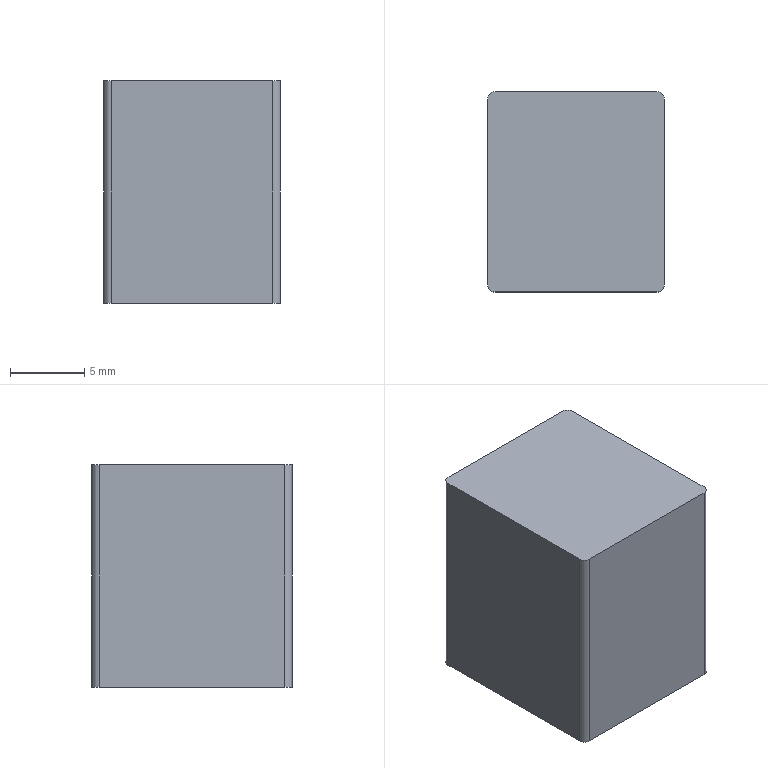Part | NX | features BREP 1 | 1 solid | 10 faces | box 11.9 x 13.498 x 15 mm | volume 2406 mm3 | plane 6 | cylinder 4 | commonest cylinder face diameters 1 x4
STEP:
#1=CARTESIAN_POINT('',(-5.45,6.749,-25.6));
#2=VERTEX_POINT('',#1);
#3=CARTESIAN_POINT('',(-5.95,6.249,-25.6));
#4=VERTEX_POINT('',#3);
#5=CARTESIAN_POINT('',(-5.45,6.249,-25.6));
#6=DIRECTION('',(0.,0.,1.));
#7=DIRECTION('',(1.,0.,0.));
#8=AXIS2_PLACEMENT_3D('',#5,#6,#7);
#9=CIRCLE('',#8,0.5);
#10=EDGE_CURVE('',#2,#4,#9,.T.);
#11=ORIENTED_EDGE('',*,*,#10,.F.);
#12=CARTESIAN_POINT('',(-5.45,6.749,-40.6));
#13=VERTEX_POINT('',#12);
#14=CARTESIAN_POINT('',(-5.45,6.749,-40.6));
#15=DIRECTION('',(0.,0.,1.));
#16=VECTOR('',#15,1000.);
#17=LINE('',#14,#16);
#18=EDGE_CURVE('',#13,#2,#17,.T.);
#19=ORIENTED_EDGE('',*,*,#18,.F.);
#20=CARTESIAN_POINT('',(-5.95,6.249,-40.6));
#21=VERTEX_POINT('',#20);
#22=CARTESIAN_POINT('',(-5.45,6.249,-40.6));
#23=DIRECTION('',(0.,0.,1.));
#24=DIRECTION('',(1.,0.,0.));
#25=AXIS2_PLACEMENT_3D('',#22,#23,#24);
#26=CIRCLE('',#25,0.5);
#27=EDGE_CURVE('',#13,#21,#26,.T.);
#28=ORIENTED_EDGE('',*,*,#27,.T.);
#29=CARTESIAN_POINT('',(-5.95,6.249,-40.6));
#30=DIRECTION('',(0.,0.,1.));
#31=VECTOR('',#30,1000.);
#32=LINE('',#29,#31);
#33=EDGE_CURVE('',#21,#4,#32,.T.);
#34=ORIENTED_EDGE('',*,*,#33,.T.);
#35=EDGE_LOOP('',(#11,#19,#28,#34));
#36=FACE_BOUND('',#35,.T.);
#37=CARTESIAN_POINT('',(-5.45,6.249,-40.6));
#38=DIRECTION('',(0.,0.,1.));
#39=DIRECTION('',(-1.,0.,0.));
#40=AXIS2_PLACEMENT_3D('',#37,#38,#39);
#41=CYLINDRICAL_SURFACE('',#40,0.5);
#42=ADVANCED_FACE('',(#36),#41,.T.);
#43=CARTESIAN_POINT('',(-5.95,-6.249,-25.6));
#44=VERTEX_POINT('',#43);
#45=CARTESIAN_POINT('',(-5.95,-6.249,-25.6));
#46=DIRECTION('',(0.,1.,0.));
#47=VECTOR('',#46,1000.);
#48=LINE('',#45,#47);
#49=EDGE_CURVE('',#44,#4,#48,.T.);
#50=ORIENTED_EDGE('',*,*,#49,.T.);
#51=ORIENTED_EDGE('',*,*,#33,.F.);
#52=CARTESIAN_POINT('',(-5.95,-6.249,-40.6));
#53=VERTEX_POINT('',#52);
#54=CARTESIAN_POINT('',(-5.95,-6.249,-40.6));
#55=DIRECTION('',(0.,1.,0.));
#56=VECTOR('',#55,1000.);
#57=LINE('',#54,#56);
#58=EDGE_CURVE('',#53,#21,#57,.T.);
#59=ORIENTED_EDGE('',*,*,#58,.F.);
#60=CARTESIAN_POINT('',(-5.95,-6.249,-40.6));
#61=DIRECTION('',(0.,0.,1.));
#62=VECTOR('',#61,1000.);
#63=LINE('',#60,#62);
#64=EDGE_CURVE('',#53,#44,#63,.T.);
#65=ORIENTED_EDGE('',*,*,#64,.T.);
#66=EDGE_LOOP('',(#50,#51,#59,#65));
#67=FACE_BOUND('',#66,.T.);
#68=CARTESIAN_POINT('',(-5.95,-6.249,-40.6));
#69=DIRECTION('',(1.,0.,0.));
#70=DIRECTION('',(0.,-1.,0.));
#71=AXIS2_PLACEMENT_3D('',#68,#69,#70);
#72=PLANE('',#71);
#73=ADVANCED_FACE('',(#67),#72,.F.);
#74=CARTESIAN_POINT('',(-5.45,-6.749,-25.6));
#75=VERTEX_POINT('',#74);
#76=CARTESIAN_POINT('',(-5.45,-6.249,-25.6));
#77=DIRECTION('',(0.,0.,1.));
#78=DIRECTION('',(1.,0.,0.));
#79=AXIS2_PLACEMENT_3D('',#76,#77,#78);
#80=CIRCLE('',#79,0.5);
#81=EDGE_CURVE('',#44,#75,#80,.T.);
#82=ORIENTED_EDGE('',*,*,#81,.F.);
#83=ORIENTED_EDGE('',*,*,#64,.F.);
#84=CARTESIAN_POINT('',(-5.45,-6.749,-40.6));
#85=VERTEX_POINT('',#84);
#86=CARTESIAN_POINT('',(-5.45,-6.249,-40.6));
#87=DIRECTION('',(0.,0.,1.));
#88=DIRECTION('',(1.,0.,0.));
#89=AXIS2_PLACEMENT_3D('',#86,#87,#88);
#90=CIRCLE('',#89,0.5);
#91=EDGE_CURVE('',#53,#85,#90,.T.);
#92=ORIENTED_EDGE('',*,*,#91,.T.);
#93=CARTESIAN_POINT('',(-5.45,-6.749,-40.6));
#94=DIRECTION('',(0.,0.,1.));
#95=VECTOR('',#94,1000.);
#96=LINE('',#93,#95);
#97=EDGE_CURVE('',#85,#75,#96,.T.);
#98=ORIENTED_EDGE('',*,*,#97,.T.);
#99=EDGE_LOOP('',(#82,#83,#92,#98));
#100=FACE_BOUND('',#99,.T.);
#101=CARTESIAN_POINT('',(-5.45,-6.249,-40.6));
#102=DIRECTION('',(0.,0.,1.));
#103=DIRECTION('',(-1.,0.,0.));
#104=AXIS2_PLACEMENT_3D('',#101,#102,#103);
#105=CYLINDRICAL_SURFACE('',#104,0.5);
#106=ADVANCED_FACE('',(#100),#105,.T.);
#107=CARTESIAN_POINT('',(5.45,-6.749,-25.6));
#108=VERTEX_POINT('',#107);
#109=CARTESIAN_POINT('',(5.45,-6.749,-25.6));
#110=DIRECTION('',(-1.,0.,0.));
#111=VECTOR('',#110,1000.);
#112=LINE('',#109,#111);
#113=EDGE_CURVE('',#108,#75,#112,.T.);
#114=ORIENTED_EDGE('',*,*,#113,.T.);
#115=ORIENTED_EDGE('',*,*,#97,.F.);
#116=CARTESIAN_POINT('',(5.45,-6.749,-40.6));
#117=VERTEX_POINT('',#116);
#118=CARTESIAN_POINT('',(5.45,-6.749,-40.6));
#119=DIRECTION('',(-1.,0.,0.));
#120=VECTOR('',#119,1000.);
#121=LINE('',#118,#120);
#122=EDGE_CURVE('',#117,#85,#121,.T.);
#123=ORIENTED_EDGE('',*,*,#122,.F.);
#124=CARTESIAN_POINT('',(5.45,-6.749,-40.6));
#125=DIRECTION('',(0.,0.,1.));
#126=VECTOR('',#125,1000.);
#127=LINE('',#124,#126);
#128=EDGE_CURVE('',#117,#108,#127,.T.);
#129=ORIENTED_EDGE('',*,*,#128,.T.);
#130=EDGE_LOOP('',(#114,#115,#123,#129));
#131=FACE_BOUND('',#130,.T.);
#132=CARTESIAN_POINT('',(5.45,-6.749,-40.6));
#133=DIRECTION('',(0.,1.,0.));
#134=DIRECTION('',(0.,0.,-1.));
#135=AXIS2_PLACEMENT_3D('',#132,#133,#134);
#136=PLANE('',#135);
#137=ADVANCED_FACE('',(#131),#136,.F.);
#138=CARTESIAN_POINT('',(5.95,-6.249,-25.6));
#139=VERTEX_POINT('',#138);
#140=CARTESIAN_POINT('',(5.45,-6.249,-25.6));
#141=DIRECTION('',(0.,0.,1.));
#142=DIRECTION('',(1.,0.,0.));
#143=AXIS2_PLACEMENT_3D('',#140,#141,#142);
#144=CIRCLE('',#143,0.5);
#145=EDGE_CURVE('',#108,#139,#144,.T.);
#146=ORIENTED_EDGE('',*,*,#145,.F.);
#147=ORIENTED_EDGE('',*,*,#128,.F.);
#148=CARTESIAN_POINT('',(5.95,-6.249,-40.6));
#149=VERTEX_POINT('',#148);
#150=CARTESIAN_POINT('',(5.45,-6.249,-40.6));
#151=DIRECTION('',(0.,0.,1.));
#152=DIRECTION('',(1.,0.,0.));
#153=AXIS2_PLACEMENT_3D('',#150,#151,#152);
#154=CIRCLE('',#153,0.5);
#155=EDGE_CURVE('',#117,#149,#154,.T.);
#156=ORIENTED_EDGE('',*,*,#155,.T.);
#157=CARTESIAN_POINT('',(5.95,-6.249,-40.6));
#158=DIRECTION('',(0.,0.,1.));
#159=VECTOR('',#158,1000.);
#160=LINE('',#157,#159);
#161=EDGE_CURVE('',#149,#139,#160,.T.);
#162=ORIENTED_EDGE('',*,*,#161,.T.);
#163=EDGE_LOOP('',(#146,#147,#156,#162));
#164=FACE_BOUND('',#163,.T.);
#165=CARTESIAN_POINT('',(5.45,-6.249,-40.6));
#166=DIRECTION('',(0.,0.,1.));
#167=DIRECTION('',(-1.,0.,0.));
#168=AXIS2_PLACEMENT_3D('',#165,#166,#167);
#169=CYLINDRICAL_SURFACE('',#168,0.5);
#170=ADVANCED_FACE('',(#164),#169,.T.);
#171=CARTESIAN_POINT('',(5.95,6.249,-25.6));
#172=VERTEX_POINT('',#171);
#173=CARTESIAN_POINT('',(5.95,6.249,-25.6));
#174=DIRECTION('',(0.,-1.,0.));
#175=VECTOR('',#174,1000.);
#176=LINE('',#173,#175);
#177=EDGE_CURVE('',#172,#139,#176,.T.);
#178=ORIENTED_EDGE('',*,*,#177,.T.);
#179=ORIENTED_EDGE('',*,*,#161,.F.);
#180=CARTESIAN_POINT('',(5.95,6.249,-40.6));
#181=VERTEX_POINT('',#180);
#182=CARTESIAN_POINT('',(5.95,6.249,-40.6));
#183=DIRECTION('',(0.,-1.,0.));
#184=VECTOR('',#183,1000.);
#185=LINE('',#182,#184);
#186=EDGE_CURVE('',#181,#149,#185,.T.);
#187=ORIENTED_EDGE('',*,*,#186,.F.);
#188=CARTESIAN_POINT('',(5.95,6.249,-40.6));
#189=DIRECTION('',(0.,0.,1.));
#190=VECTOR('',#189,1000.);
#191=LINE('',#188,#190);
#192=EDGE_CURVE('',#181,#172,#191,.T.);
#193=ORIENTED_EDGE('',*,*,#192,.T.);
#194=EDGE_LOOP('',(#178,#179,#187,#193));
#195=FACE_BOUND('',#194,.T.);
#196=CARTESIAN_POINT('',(5.95,6.249,-40.6));
#197=DIRECTION('',(-1.,0.,0.));
#198=DIRECTION('',(0.,1.,0.));
#199=AXIS2_PLACEMENT_3D('',#196,#197,#198);
#200=PLANE('',#199);
#201=ADVANCED_FACE('',(#195),#200,.F.);
#202=CARTESIAN_POINT('',(5.45,6.749,-25.6));
#203=VERTEX_POINT('',#202);
#204=CARTESIAN_POINT('',(5.45,6.249,-25.6));
#205=DIRECTION('',(0.,0.,1.));
#206=DIRECTION('',(1.,0.,0.));
#207=AXIS2_PLACEMENT_3D('',#204,#205,#206);
#208=CIRCLE('',#207,0.5);
#209=EDGE_CURVE('',#172,#203,#208,.T.);
#210=ORIENTED_EDGE('',*,*,#209,.F.);
#211=ORIENTED_EDGE('',*,*,#192,.F.);
#212=CARTESIAN_POINT('',(5.45,6.749,-40.6));
#213=VERTEX_POINT('',#212);
#214=CARTESIAN_POINT('',(5.45,6.249,-40.6));
#215=DIRECTION('',(0.,0.,1.));
#216=DIRECTION('',(1.,0.,0.));
#217=AXIS2_PLACEMENT_3D('',#214,#215,#216);
#218=CIRCLE('',#217,0.5);
#219=EDGE_CURVE('',#181,#213,#218,.T.);
#220=ORIENTED_EDGE('',*,*,#219,.T.);
#221=CARTESIAN_POINT('',(5.45,6.749,-40.6));
#222=DIRECTION('',(0.,0.,1.));
#223=VECTOR('',#222,1000.);
#224=LINE('',#221,#223);
#225=EDGE_CURVE('',#213,#203,#224,.T.);
#226=ORIENTED_EDGE('',*,*,#225,.T.);
#227=EDGE_LOOP('',(#210,#211,#220,#226));
#228=FACE_BOUND('',#227,.T.);
#229=CARTESIAN_POINT('',(5.45,6.249,-40.6));
#230=DIRECTION('',(0.,0.,1.));
#231=DIRECTION('',(-1.,0.,0.));
#232=AXIS2_PLACEMENT_3D('',#229,#230,#231);
#233=CYLINDRICAL_SURFACE('',#232,0.5);
#234=ADVANCED_FACE('',(#228),#233,.T.);
#235=CARTESIAN_POINT('',(-5.45,6.749,-25.6));
#236=DIRECTION('',(1.,0.,0.));
#237=VECTOR('',#236,1000.);
#238=LINE('',#235,#237);
#239=EDGE_CURVE('',#2,#203,#238,.T.);
#240=ORIENTED_EDGE('',*,*,#239,.T.);
#241=ORIENTED_EDGE('',*,*,#225,.F.);
#242=CARTESIAN_POINT('',(-5.45,6.749,-40.6));
#243=DIRECTION('',(1.,0.,0.));
#244=VECTOR('',#243,1000.);
#245=LINE('',#242,#244);
#246=EDGE_CURVE('',#13,#213,#245,.T.);
#247=ORIENTED_EDGE('',*,*,#246,.F.);
#248=ORIENTED_EDGE('',*,*,#18,.T.);
#249=EDGE_LOOP('',(#240,#241,#247,#248));
#250=FACE_BOUND('',#249,.T.);
#251=CARTESIAN_POINT('',(-5.45,6.749,-40.6));
#252=DIRECTION('',(0.,-1.,0.));
#253=DIRECTION('',(0.,0.,1.));
#254=AXIS2_PLACEMENT_3D('',#251,#252,#253);
#255=PLANE('',#254);
#256=ADVANCED_FACE('',(#250),#255,.F.);
#257=ORIENTED_EDGE('',*,*,#27,.F.);
#258=ORIENTED_EDGE('',*,*,#246,.T.);
#259=ORIENTED_EDGE('',*,*,#219,.F.);
#260=ORIENTED_EDGE('',*,*,#186,.T.);
#261=ORIENTED_EDGE('',*,*,#155,.F.);
#262=ORIENTED_EDGE('',*,*,#122,.T.);
#263=ORIENTED_EDGE('',*,*,#91,.F.);
#264=ORIENTED_EDGE('',*,*,#58,.T.);
#265=EDGE_LOOP('',(#257,#258,#259,#260,#261,#262,#263,#264));
#266=FACE_BOUND('',#265,.T.);
#267=CARTESIAN_POINT('',(-5.45,6.249,-40.6));
#268=DIRECTION('',(0.,0.,1.));
#269=DIRECTION('',(-1.,0.,0.));
#270=AXIS2_PLACEMENT_3D('',#267,#268,#269);
#271=PLANE('',#270);
#272=ADVANCED_FACE('',(#266),#271,.F.);
#273=ORIENTED_EDGE('',*,*,#10,.T.);
#274=ORIENTED_EDGE('',*,*,#49,.F.);
#275=ORIENTED_EDGE('',*,*,#81,.T.);
#276=ORIENTED_EDGE('',*,*,#113,.F.);
#277=ORIENTED_EDGE('',*,*,#145,.T.);
#278=ORIENTED_EDGE('',*,*,#177,.F.);
#279=ORIENTED_EDGE('',*,*,#209,.T.);
#280=ORIENTED_EDGE('',*,*,#239,.F.);
#281=EDGE_LOOP('',(#273,#274,#275,#276,#277,#278,#279,#280));
#282=FACE_BOUND('',#281,.T.);
#283=CARTESIAN_POINT('',(-5.45,6.249,-25.6));
#284=DIRECTION('',(0.,0.,1.));
#285=DIRECTION('',(-1.,0.,0.));
#286=AXIS2_PLACEMENT_3D('',#283,#284,#285);
#287=PLANE('',#286);
#288=ADVANCED_FACE('',(#282),#287,.T.);
#289=CLOSED_SHELL('',(#42,#73,#106,#137,#170,#201,#234,#256,#272,#288));
#290=MANIFOLD_SOLID_BREP('',#289);
#291=(LENGTH_UNIT()NAMED_UNIT(*)SI_UNIT(.MILLI.,.METRE.));
#292=UNCERTAINTY_MEASURE_WITH_UNIT(LENGTH_MEASURE(0.00001),#291,'','');
#293=(NAMED_UNIT(*)PLANE_ANGLE_UNIT()SI_UNIT($,.RADIAN.));
#294=(NAMED_UNIT(*)SI_UNIT($,.STERADIAN.)SOLID_ANGLE_UNIT());
#295=(GEOMETRIC_REPRESENTATION_CONTEXT(3)GLOBAL_UNCERTAINTY_ASSIGNED_CONTEXT((#292))GLOBAL_UNIT_ASSIGNED_CONTEXT((#291,#293,#294))REPRESENTATION_CONTEXT('',''));
#296=ADVANCED_BREP_SHAPE_REPRESENTATION('',(#290),#295);